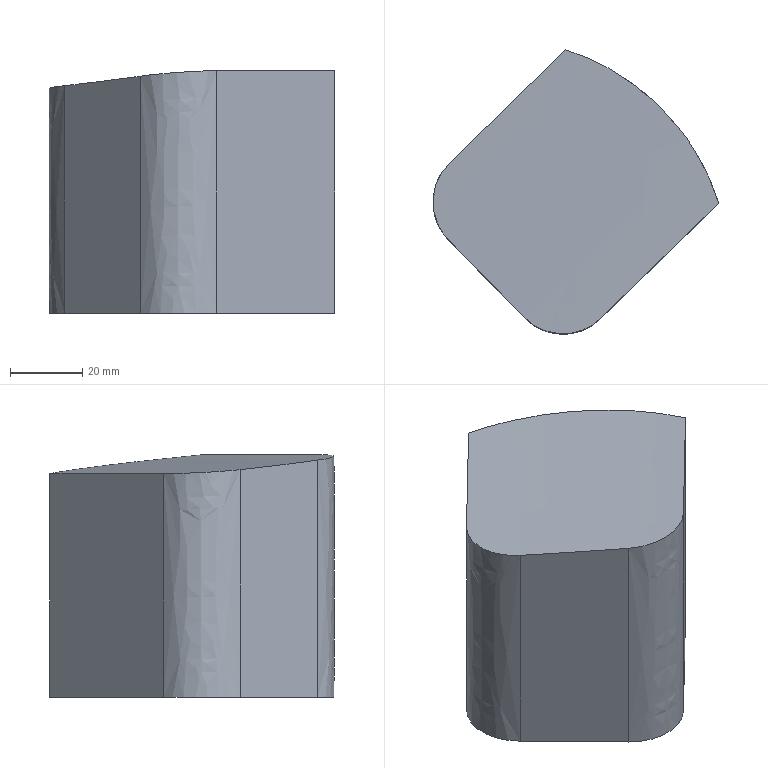Part | NX | features solid 2 | 1 solid | 10 faces | box 79.06 x 78.572 x 67.121 mm | volume 243616 mm3 | spline 6 | plane 2 | cylinder 1 | cone 1 | commonest cylinder face diameters 10 x1
STEP:
#1=CARTESIAN_POINT('',(-262.435,327.996,-28.));
#2=VERTEX_POINT('',#1);
#3=CARTESIAN_POINT('',(-283.378,349.476,-28.));
#4=VERTEX_POINT('',#3);
#5=CARTESIAN_POINT('',(-126.138,188.203,-28.));
#6=DIRECTION('',(0.6981,-0.716,0.));
#7=VECTOR('',#6,1000.);
#8=LINE('',#5,#7);
#9=EDGE_CURVE('',#2,#4,#8,.F.);
#10=ORIENTED_EDGE('',*,*,#9,.T.);
#11=CARTESIAN_POINT('',(-283.11,370.687,-28.));
#12=VERTEX_POINT('',#11);
#13=CARTESIAN_POINT('',(-272.638,359.947,-28.));
#14=DIRECTION('',(0.,0.,1.));
#15=DIRECTION('',(1.,0.,0.));
#16=AXIS2_PLACEMENT_3D('',#13,#14,#15);
#17=CIRCLE('',#16,15.);
#18=EDGE_CURVE('',#4,#12,#17,.F.);
#19=ORIENTED_EDGE('',*,*,#18,.T.);
#20=CARTESIAN_POINT('',(-250.953,402.04,-28.));
#21=VERTEX_POINT('',#20);
#22=CARTESIAN_POINT('',(-283.11,370.687,-28.));
#23=CARTESIAN_POINT('',(-272.391,381.138,-28.));
#24=CARTESIAN_POINT('',(-261.672,391.589,-28.));
#25=CARTESIAN_POINT('',(-250.953,402.04,-28.));
#26=B_SPLINE_CURVE_WITH_KNOTS('',3,(#22,#23,#24,#25),.UNSPECIFIED.,.F.,.F.,(4,4),(0.,1.),.UNSPECIFIED.);
#27=EDGE_CURVE('',#21,#12,#26,.F.);
#28=ORIENTED_EDGE('',*,*,#27,.F.);
#29=CARTESIAN_POINT('',(-208.578,359.557,-28.));
#30=VERTEX_POINT('',#29);
#31=CARTESIAN_POINT('',(-250.953,402.04,-28.));
#32=CARTESIAN_POINT('',(-246.004,400.47,-28.));
#33=CARTESIAN_POINT('',(-236.524,396.138,-28.));
#34=CARTESIAN_POINT('',(-220.033,383.168,-28.));
#35=CARTESIAN_POINT('',(-211.698,369.488,-28.));
#36=CARTESIAN_POINT('',(-208.578,359.557,-28.));
#37=B_SPLINE_CURVE_WITH_KNOTS('',3,(#31,#32,#33,#34,#35,#36),.UNSPECIFIED.,.F.,.F.,(4,1,1,4),(0.,0.25,0.5,1.),.UNSPECIFIED.);
#38=EDGE_CURVE('',#21,#30,#37,.T.);
#39=ORIENTED_EDGE('',*,*,#38,.T.);
#40=CARTESIAN_POINT('',(-241.224,327.727,-28.));
#41=VERTEX_POINT('',#40);
#42=CARTESIAN_POINT('',(-208.578,359.557,-28.));
#43=CARTESIAN_POINT('',(-219.46,348.947,-28.));
#44=CARTESIAN_POINT('',(-230.342,338.337,-28.));
#45=CARTESIAN_POINT('',(-241.224,327.727,-28.));
#46=B_SPLINE_CURVE_WITH_KNOTS('',3,(#42,#43,#44,#45),.UNSPECIFIED.,.F.,.F.,(4,4),(0.,1.),.UNSPECIFIED.);
#47=EDGE_CURVE('',#30,#41,#46,.T.);
#48=ORIENTED_EDGE('',*,*,#47,.T.);
#49=CARTESIAN_POINT('',(-251.695,338.467,-28.));
#50=DIRECTION('',(0.,0.,1.));
#51=DIRECTION('',(1.,0.,0.));
#52=AXIS2_PLACEMENT_3D('',#49,#50,#51);
#53=CIRCLE('',#52,15.);
#54=EDGE_CURVE('',#41,#2,#53,.F.);
#55=ORIENTED_EDGE('',*,*,#54,.T.);
#56=EDGE_LOOP('',(#10,#19,#28,#39,#48,#55));
#57=FACE_BOUND('',#56,.T.);
#58=CARTESIAN_POINT('',(-246.427,359.679,-28.));
#59=VERTEX_POINT('',#58);
#60=CARTESIAN_POINT('',(-251.427,359.679,-28.));
#61=DIRECTION('',(0.,0.,1.));
#62=DIRECTION('',(1.,0.,0.));
#63=AXIS2_PLACEMENT_3D('',#60,#61,#62);
#64=CIRCLE('',#63,5.);
#65=EDGE_CURVE('',#59,#59,#64,.T.);
#66=ORIENTED_EDGE('',*,*,#65,.T.);
#67=EDGE_LOOP('',(#66));
#68=FACE_BOUND('',#67,.T.);
#69=CARTESIAN_POINT('',(-252.5,65.,-28.));
#70=DIRECTION('',(0.,0.,1.));
#71=DIRECTION('',(-1.,0.,0.));
#72=AXIS2_PLACEMENT_3D('',#69,#70,#71);
#73=PLANE('',#72);
#74=ADVANCED_FACE('',(#57,#68),#73,.F.);
#75=CARTESIAN_POINT('',(-208.578,359.557,39.121));
#76=VERTEX_POINT('',#75);
#77=CARTESIAN_POINT('',(-241.224,327.727,39.121));
#78=VERTEX_POINT('',#77);
#79=CARTESIAN_POINT('',(-208.578,359.557,39.121));
#80=CARTESIAN_POINT('',(-219.46,348.947,39.121));
#81=CARTESIAN_POINT('',(-230.342,338.337,39.121));
#82=CARTESIAN_POINT('',(-241.224,327.727,39.121));
#83=B_SPLINE_CURVE_WITH_KNOTS('',3,(#79,#80,#81,#82),.UNSPECIFIED.,.F.,.F.,(4,4),(0.07628,0.1219),.UNSPECIFIED.);
#84=EDGE_CURVE('',#76,#78,#83,.T.);
#85=ORIENTED_EDGE('',*,*,#84,.T.);
#86=CARTESIAN_POINT('',(-241.224,327.727,39.121));
#87=CARTESIAN_POINT('',(-241.224,327.727,16.747));
#88=CARTESIAN_POINT('',(-241.224,327.727,-5.626));
#89=CARTESIAN_POINT('',(-241.224,327.727,-28.));
#90=B_SPLINE_CURVE_WITH_KNOTS('',3,(#86,#87,#88,#89),.UNSPECIFIED.,.F.,.F.,(4,4),(0.,0.06712),.UNSPECIFIED.);
#91=EDGE_CURVE('',#78,#41,#90,.T.);
#92=ORIENTED_EDGE('',*,*,#91,.T.);
#93=ORIENTED_EDGE('',*,*,#47,.F.);
#94=CARTESIAN_POINT('',(-208.578,359.557,-28.));
#95=CARTESIAN_POINT('',(-208.578,359.557,-5.626));
#96=CARTESIAN_POINT('',(-208.578,359.557,16.747));
#97=CARTESIAN_POINT('',(-208.578,359.557,39.121));
#98=B_SPLINE_CURVE_WITH_KNOTS('',3,(#94,#95,#96,#97),.UNSPECIFIED.,.F.,.F.,(4,4),(0.185,0.2521),.UNSPECIFIED.);
#99=EDGE_CURVE('',#30,#76,#98,.T.);
#100=ORIENTED_EDGE('',*,*,#99,.T.);
#101=EDGE_LOOP('',(#85,#92,#93,#100));
#102=FACE_BOUND('',#101,.T.);
#103=CARTESIAN_POINT('',(-241.224,327.727,-28.));
#104=CARTESIAN_POINT('',(-241.224,327.727,-5.626));
#105=CARTESIAN_POINT('',(-241.224,327.727,16.747));
#106=CARTESIAN_POINT('',(-241.224,327.727,39.121));
#107=CARTESIAN_POINT('',(-230.342,338.337,-28.));
#108=CARTESIAN_POINT('',(-230.342,338.337,-5.626));
#109=CARTESIAN_POINT('',(-230.342,338.337,16.747));
#110=CARTESIAN_POINT('',(-230.342,338.337,39.121));
#111=CARTESIAN_POINT('',(-219.46,348.947,-28.));
#112=CARTESIAN_POINT('',(-219.46,348.947,-5.626));
#113=CARTESIAN_POINT('',(-219.46,348.947,16.747));
#114=CARTESIAN_POINT('',(-219.46,348.947,39.121));
#115=CARTESIAN_POINT('',(-208.578,359.557,-28.));
#116=CARTESIAN_POINT('',(-208.578,359.557,-5.626));
#117=CARTESIAN_POINT('',(-208.578,359.557,16.747));
#118=CARTESIAN_POINT('',(-208.578,359.557,39.121));
#119=B_SPLINE_SURFACE_WITH_KNOTS('',3,3,((#103,#104,#105,#106),(#107,#108,#109,#110),(#111,#112,#113,#114),(#115,#116,#117,#118)),.UNSPECIFIED.,.F.,.F.,.F.,(4,4),(4,4),(0.3532,0.6878),(0.3333,0.9491),.UNSPECIFIED.);
#120=ADVANCED_FACE('',(#102),#119,.T.);
#121=ORIENTED_EDGE('',*,*,#27,.T.);
#122=CARTESIAN_POINT('',(-283.11,370.687,33.895));
#123=VERTEX_POINT('',#122);
#124=CARTESIAN_POINT('',(-283.11,370.687,-28.));
#125=CARTESIAN_POINT('',(-283.11,370.687,-7.368));
#126=CARTESIAN_POINT('',(-283.11,370.687,13.263));
#127=CARTESIAN_POINT('',(-283.11,370.687,33.895));
#128=B_SPLINE_CURVE_WITH_KNOTS('',3,(#124,#125,#126,#127),.UNSPECIFIED.,.F.,.F.,(4,4),(0.,0.06189),.UNSPECIFIED.);
#129=EDGE_CURVE('',#12,#123,#128,.T.);
#130=ORIENTED_EDGE('',*,*,#129,.T.);
#131=CARTESIAN_POINT('',(-250.953,402.04,33.895));
#132=VERTEX_POINT('',#131);
#133=CARTESIAN_POINT('',(-250.953,402.04,33.895));
#134=CARTESIAN_POINT('',(-261.672,391.589,33.895));
#135=CARTESIAN_POINT('',(-272.391,381.138,33.895));
#136=CARTESIAN_POINT('',(-283.11,370.687,33.895));
#137=B_SPLINE_CURVE_WITH_KNOTS('',3,(#133,#134,#135,#136),.UNSPECIFIED.,.F.,.F.,(4,4),(0.222,0.2669),.UNSPECIFIED.);
#138=EDGE_CURVE('',#132,#123,#137,.T.);
#139=ORIENTED_EDGE('',*,*,#138,.F.);
#140=CARTESIAN_POINT('',(-250.953,402.04,-28.));
#141=CARTESIAN_POINT('',(-250.953,402.04,-7.368));
#142=CARTESIAN_POINT('',(-250.953,402.04,13.263));
#143=CARTESIAN_POINT('',(-250.953,402.04,33.895));
#144=B_SPLINE_CURVE_WITH_KNOTS('',3,(#140,#141,#142,#143),.UNSPECIFIED.,.F.,.F.,(4,4),(0.185,0.2468),.UNSPECIFIED.);
#145=EDGE_CURVE('',#21,#132,#144,.T.);
#146=ORIENTED_EDGE('',*,*,#145,.F.);
#147=EDGE_LOOP('',(#121,#130,#139,#146));
#148=FACE_BOUND('',#147,.T.);
#149=CARTESIAN_POINT('',(-283.11,370.687,33.895));
#150=CARTESIAN_POINT('',(-272.391,381.138,33.895));
#151=CARTESIAN_POINT('',(-261.672,391.589,33.895));
#152=CARTESIAN_POINT('',(-250.953,402.04,33.895));
#153=CARTESIAN_POINT('',(-283.11,370.687,13.263));
#154=CARTESIAN_POINT('',(-272.391,381.138,13.263));
#155=CARTESIAN_POINT('',(-261.672,391.589,13.263));
#156=CARTESIAN_POINT('',(-250.953,402.04,13.263));
#157=CARTESIAN_POINT('',(-283.11,370.687,-7.368));
#158=CARTESIAN_POINT('',(-272.391,381.138,-7.368));
#159=CARTESIAN_POINT('',(-261.672,391.589,-7.368));
#160=CARTESIAN_POINT('',(-250.953,402.04,-7.368));
#161=CARTESIAN_POINT('',(-283.11,370.687,-28.));
#162=CARTESIAN_POINT('',(-272.391,381.138,-28.));
#163=CARTESIAN_POINT('',(-261.672,391.589,-28.));
#164=CARTESIAN_POINT('',(-250.953,402.04,-28.));
#165=B_SPLINE_SURFACE_WITH_KNOTS('',3,3,((#149,#150,#151,#152),(#153,#154,#155,#156),(#157,#158,#159,#160),(#161,#162,#163,#164)),.UNSPECIFIED.,.F.,.F.,.F.,(4,4),(4,4),(0.1216,0.6667),(0.3541,0.699),.UNSPECIFIED.);
#166=ADVANCED_FACE('',(#148),#165,.F.);
#167=ORIENTED_EDGE('',*,*,#138,.T.);
#168=CARTESIAN_POINT('',(-283.378,349.476,34.974));
#169=VERTEX_POINT('',#168);
#170=CARTESIAN_POINT('',(-283.11,370.687,33.895));
#171=CARTESIAN_POINT('',(-284.53,369.303,33.895));
#172=CARTESIAN_POINT('',(-286.778,366.015,33.945));
#173=CARTESIAN_POINT('',(-288.452,358.167,34.244));
#174=CARTESIAN_POINT('',(-286.139,352.307,34.666));
#175=CARTESIAN_POINT('',(-283.378,349.476,34.974));
#176=B_SPLINE_CURVE_WITH_KNOTS('',3,(#170,#171,#172,#173,#174,#175),.UNSPECIFIED.,.F.,.F.,(4,1,1,4),(0.,0.005866,0.01173,0.02346),.UNSPECIFIED.);
#177=EDGE_CURVE('',#123,#169,#176,.T.);
#178=ORIENTED_EDGE('',*,*,#177,.T.);
#179=CARTESIAN_POINT('',(-262.435,327.996,37.604));
#180=VERTEX_POINT('',#179);
#181=CARTESIAN_POINT('',(-283.378,349.476,34.974));
#182=CARTESIAN_POINT('',(-276.391,342.31,35.753));
#183=CARTESIAN_POINT('',(-269.41,335.15,36.637));
#184=CARTESIAN_POINT('',(-262.435,327.996,37.604));
#185=B_SPLINE_CURVE_WITH_KNOTS('',3,(#181,#182,#183,#184),.UNSPECIFIED.,.F.,.F.,(4,4),(0.06969,0.09858),.UNSPECIFIED.);
#186=EDGE_CURVE('',#169,#180,#185,.T.);
#187=ORIENTED_EDGE('',*,*,#186,.T.);
#188=CARTESIAN_POINT('',(-262.435,327.996,37.604));
#189=CARTESIAN_POINT('',(-261.055,326.581,37.795));
#190=CARTESIAN_POINT('',(-257.782,324.338,38.178));
#191=CARTESIAN_POINT('',(-249.952,322.65,38.858));
#192=CARTESIAN_POINT('',(-244.068,324.954,39.121));
#193=CARTESIAN_POINT('',(-241.224,327.727,39.121));
#194=B_SPLINE_CURVE_WITH_KNOTS('',3,(#188,#189,#190,#191,#192,#193),.UNSPECIFIED.,.F.,.F.,(4,1,1,4),(0.,0.005873,0.01175,0.02349),.UNSPECIFIED.);
#195=EDGE_CURVE('',#180,#78,#194,.T.);
#196=ORIENTED_EDGE('',*,*,#195,.T.);
#197=ORIENTED_EDGE('',*,*,#84,.F.);
#198=CARTESIAN_POINT('',(-208.578,359.557,39.121));
#199=CARTESIAN_POINT('',(-210.141,364.533,38.628));
#200=CARTESIAN_POINT('',(-213.339,371.584,37.89));
#201=CARTESIAN_POINT('',(-219.316,380.234,36.907));
#202=CARTESIAN_POINT('',(-224.462,386.046,36.207));
#203=CARTESIAN_POINT('',(-230.272,391.225,35.544));
#204=CARTESIAN_POINT('',(-238.907,397.232,34.717));
#205=CARTESIAN_POINT('',(-245.958,400.456,34.197));
#206=CARTESIAN_POINT('',(-250.953,402.04,33.895));
#207=B_SPLINE_CURVE_WITH_KNOTS('',3,(#198,#199,#200,#201,#202,#203,#204,#205,#206),.UNSPECIFIED.,.F.,.F.,(4,1,1,1,1,1,4),(0.03682,0.05232,0.06007,0.06781,0.07556,0.08331,0.09881),.UNSPECIFIED.);
#208=EDGE_CURVE('',#76,#132,#207,.T.);
#209=ORIENTED_EDGE('',*,*,#208,.T.);
#210=EDGE_LOOP('',(#167,#178,#187,#196,#197,#209));
#211=FACE_BOUND('',#210,.T.);
#212=CARTESIAN_POINT('',(-299.649,354.562,33.895));
#213=CARTESIAN_POINT('',(-250.658,402.328,33.895));
#214=CARTESIAN_POINT('',(-289.727,351.41,34.495));
#215=CARTESIAN_POINT('',(-240.735,399.177,34.495));
#216=CARTESIAN_POINT('',(-271.485,340.225,36.109));
#217=CARTESIAN_POINT('',(-222.494,387.991,36.109));
#218=CARTESIAN_POINT('',(-260.394,321.981,38.14));
#219=CARTESIAN_POINT('',(-211.403,369.747,38.14));
#220=CARTESIAN_POINT('',(-257.275,312.078,39.121));
#221=CARTESIAN_POINT('',(-208.283,359.844,39.121));
#222=B_SPLINE_SURFACE_WITH_KNOTS('',3,1,((#212,#213),(#214,#215),(#216,#217),(#218,#219),(#220,#221)),.SURF_OF_LINEAR_EXTRUSION.,.F.,.F.,.F.,(4,1,4),(2,2),(0.4187,0.5678,0.7168),(0.,1.),.UNSPECIFIED.);
#223=ADVANCED_FACE('',(#211),#222,.T.);
#224=ORIENTED_EDGE('',*,*,#99,.F.);
#225=ORIENTED_EDGE('',*,*,#38,.F.);
#226=ORIENTED_EDGE('',*,*,#145,.T.);
#227=ORIENTED_EDGE('',*,*,#208,.F.);
#228=EDGE_LOOP('',(#224,#225,#226,#227));
#229=FACE_BOUND('',#228,.T.);
#230=CARTESIAN_POINT('',(-208.578,359.557,-28.));
#231=CARTESIAN_POINT('',(-208.578,359.557,39.524));
#232=CARTESIAN_POINT('',(-211.69,369.461,-28.));
#233=CARTESIAN_POINT('',(-211.69,369.461,39.524));
#234=CARTESIAN_POINT('',(-222.792,387.711,-28.));
#235=CARTESIAN_POINT('',(-222.792,387.711,39.524));
#236=CARTESIAN_POINT('',(-241.032,398.893,-28.));
#237=CARTESIAN_POINT('',(-241.032,398.893,39.524));
#238=CARTESIAN_POINT('',(-250.953,402.04,-28.));
#239=CARTESIAN_POINT('',(-250.953,402.04,39.524));
#240=B_SPLINE_SURFACE_WITH_KNOTS('',3,1,((#230,#231),(#232,#233),(#234,#235),(#236,#237),(#238,#239)),.SURF_OF_LINEAR_EXTRUSION.,.F.,.F.,.F.,(4,1,4),(2,2),(0.1514,0.1645,0.1776),(0.,1.),.UNSPECIFIED.);
#241=ADVANCED_FACE('',(#229),#240,.T.);
#242=ORIENTED_EDGE('',*,*,#186,.F.);
#243=CARTESIAN_POINT('',(-283.378,349.476,34.974));
#244=CARTESIAN_POINT('',(-283.378,349.476,13.983));
#245=CARTESIAN_POINT('',(-283.378,349.476,-7.009));
#246=CARTESIAN_POINT('',(-283.378,349.476,-28.));
#247=B_SPLINE_CURVE_WITH_KNOTS('',3,(#243,#244,#245,#246),.UNSPECIFIED.,.F.,.F.,(4,4),(0.,0.06297),.UNSPECIFIED.);
#248=EDGE_CURVE('',#169,#4,#247,.T.);
#249=ORIENTED_EDGE('',*,*,#248,.T.);
#250=ORIENTED_EDGE('',*,*,#9,.F.);
#251=CARTESIAN_POINT('',(-262.435,327.996,-28.));
#252=CARTESIAN_POINT('',(-262.435,327.996,-6.132));
#253=CARTESIAN_POINT('',(-262.435,327.996,15.736));
#254=CARTESIAN_POINT('',(-262.435,327.996,37.604));
#255=B_SPLINE_CURVE_WITH_KNOTS('',3,(#251,#252,#253,#254),.UNSPECIFIED.,.F.,.F.,(4,4),(0.,0.0656),.UNSPECIFIED.);
#256=EDGE_CURVE('',#2,#180,#255,.T.);
#257=ORIENTED_EDGE('',*,*,#256,.T.);
#258=EDGE_LOOP('',(#242,#249,#250,#257));
#259=FACE_BOUND('',#258,.T.);
#260=CARTESIAN_POINT('',(-252.097,317.393,-18.));
#261=DIRECTION('',(-0.716,-0.6981,0.));
#262=DIRECTION('',(-0.6981,0.716,0.));
#263=AXIS2_PLACEMENT_3D('',#260,#261,#262);
#264=PLANE('',#263);
#265=ADVANCED_FACE('',(#259),#264,.T.);
#266=ORIENTED_EDGE('',*,*,#65,.F.);
#267=EDGE_LOOP('',(#266));
#268=FACE_BOUND('',#267,.T.);
#269=CARTESIAN_POINT('',(-246.427,359.679,-7.5));
#270=VERTEX_POINT('',#269);
#271=CARTESIAN_POINT('',(-251.427,359.679,-7.5));
#272=DIRECTION('',(0.,0.,1.));
#273=DIRECTION('',(1.,0.,0.));
#274=AXIS2_PLACEMENT_3D('',#271,#272,#273);
#275=CIRCLE('',#274,5.);
#276=EDGE_CURVE('',#270,#270,#275,.T.);
#277=ORIENTED_EDGE('',*,*,#276,.T.);
#278=EDGE_LOOP('',(#277));
#279=FACE_BOUND('',#278,.T.);
#280=CARTESIAN_POINT('',(-251.427,359.679,-52.5));
#281=DIRECTION('',(0.,0.,1.));
#282=DIRECTION('',(1.,0.,0.));
#283=AXIS2_PLACEMENT_3D('',#280,#281,#282);
#284=CYLINDRICAL_SURFACE('',#283,5.);
#285=ADVANCED_FACE('',(#268,#279),#284,.F.);
#286=ORIENTED_EDGE('',*,*,#276,.F.);
#287=EDGE_LOOP('',(#286));
#288=FACE_BOUND('',#287,.T.);
#289=CARTESIAN_POINT('',(-251.427,359.679,-4.496));
#290=VERTEX_POINT('',#289);
#291=VERTEX_LOOP('',#290);
#292=FACE_BOUND('',#291,.T.);
#293=CARTESIAN_POINT('',(-251.427,359.679,-7.5));
#294=DIRECTION('',(0.,0.,-1.));
#295=DIRECTION('',(-1.,0.,0.));
#296=AXIS2_PLACEMENT_3D('',#293,#294,#295);
#297=CONICAL_SURFACE('',#296,5.,1.03);
#298=ADVANCED_FACE('',(#288,#292),#297,.F.);
#299=ORIENTED_EDGE('',*,*,#18,.F.);
#300=ORIENTED_EDGE('',*,*,#248,.F.);
#301=ORIENTED_EDGE('',*,*,#177,.F.);
#302=ORIENTED_EDGE('',*,*,#129,.F.);
#303=EDGE_LOOP('',(#299,#300,#301,#302));
#304=FACE_BOUND('',#303,.T.);
#305=CARTESIAN_POINT('',(-283.11,370.687,35.352));
#306=CARTESIAN_POINT('',(-293.85,360.216,35.352));
#307=CARTESIAN_POINT('',(-283.378,349.476,35.352));
#308=CARTESIAN_POINT('',(-283.11,370.687,14.235));
#309=CARTESIAN_POINT('',(-293.85,360.216,14.235));
#310=CARTESIAN_POINT('',(-283.378,349.476,14.235));
#311=CARTESIAN_POINT('',(-283.11,370.687,-6.883));
#312=CARTESIAN_POINT('',(-293.85,360.216,-6.883));
#313=CARTESIAN_POINT('',(-283.378,349.476,-6.883));
#314=CARTESIAN_POINT('',(-283.11,370.687,-28.));
#315=CARTESIAN_POINT('',(-293.85,360.216,-28.));
#316=CARTESIAN_POINT('',(-283.378,349.476,-28.));
#317=(BOUNDED_SURFACE()B_SPLINE_SURFACE(3,2,((#305,#306,#307),(#308,#309,#310),(#311,#312,#313),(#314,#315,#316)),.UNSPECIFIED.,.F.,.F.,.F.)B_SPLINE_SURFACE_WITH_KNOTS((4,4),(3,3),(0.1379,0.2013),(0.,1.),.PIECEWISE_BEZIER_KNOTS.)GEOMETRIC_REPRESENTATION_ITEM()RATIONAL_B_SPLINE_SURFACE(((1.,0.7071,1.),(1.,0.7071,1.),(1.,0.7071,1.),(1.,0.7071,1.)))REPRESENTATION_ITEM('')SURFACE());
#318=ADVANCED_FACE('',(#304),#317,.T.);
#319=ORIENTED_EDGE('',*,*,#195,.F.);
#320=ORIENTED_EDGE('',*,*,#256,.F.);
#321=ORIENTED_EDGE('',*,*,#54,.F.);
#322=ORIENTED_EDGE('',*,*,#91,.F.);
#323=EDGE_LOOP('',(#319,#320,#321,#322));
#324=FACE_BOUND('',#323,.T.);
#325=CARTESIAN_POINT('',(-262.435,327.996,39.524));
#326=CARTESIAN_POINT('',(-251.964,317.256,39.524));
#327=CARTESIAN_POINT('',(-241.224,327.727,39.524));
#328=CARTESIAN_POINT('',(-262.435,327.996,17.016));
#329=CARTESIAN_POINT('',(-251.964,317.256,17.016));
#330=CARTESIAN_POINT('',(-241.224,327.727,17.016));
#331=CARTESIAN_POINT('',(-262.435,327.996,-5.492));
#332=CARTESIAN_POINT('',(-251.964,317.256,-5.492));
#333=CARTESIAN_POINT('',(-241.224,327.727,-5.492));
#334=CARTESIAN_POINT('',(-262.435,327.996,-28.));
#335=CARTESIAN_POINT('',(-251.964,317.256,-28.));
#336=CARTESIAN_POINT('',(-241.224,327.727,-28.));
#337=(BOUNDED_SURFACE()B_SPLINE_SURFACE(3,2,((#325,#326,#327),(#328,#329,#330),(#331,#332,#333),(#334,#335,#336)),.UNSPECIFIED.,.F.,.F.,.F.)B_SPLINE_SURFACE_WITH_KNOTS((4,4),(3,3),(0.1359,0.2034),(0.,1.),.PIECEWISE_BEZIER_KNOTS.)GEOMETRIC_REPRESENTATION_ITEM()RATIONAL_B_SPLINE_SURFACE(((1.,0.7071,1.),(1.,0.7071,1.),(1.,0.7071,1.),(1.,0.7071,1.)))REPRESENTATION_ITEM('')SURFACE());
#338=ADVANCED_FACE('',(#324),#337,.T.);
#339=CLOSED_SHELL('',(#74,#120,#166,#223,#241,#265,#285,#298,#318,#338));
#340=MANIFOLD_SOLID_BREP('',#339);
#341=(LENGTH_UNIT()NAMED_UNIT(*)SI_UNIT(.MILLI.,.METRE.));
#342=UNCERTAINTY_MEASURE_WITH_UNIT(LENGTH_MEASURE(0.0508),#341,'','');
#343=(NAMED_UNIT(*)PLANE_ANGLE_UNIT()SI_UNIT($,.RADIAN.));
#344=(NAMED_UNIT(*)SI_UNIT($,.STERADIAN.)SOLID_ANGLE_UNIT());
#345=(GEOMETRIC_REPRESENTATION_CONTEXT(3)GLOBAL_UNCERTAINTY_ASSIGNED_CONTEXT((#342))GLOBAL_UNIT_ASSIGNED_CONTEXT((#341,#343,#344))REPRESENTATION_CONTEXT('',''));
#346=ADVANCED_BREP_SHAPE_REPRESENTATION('',(#340),#345);